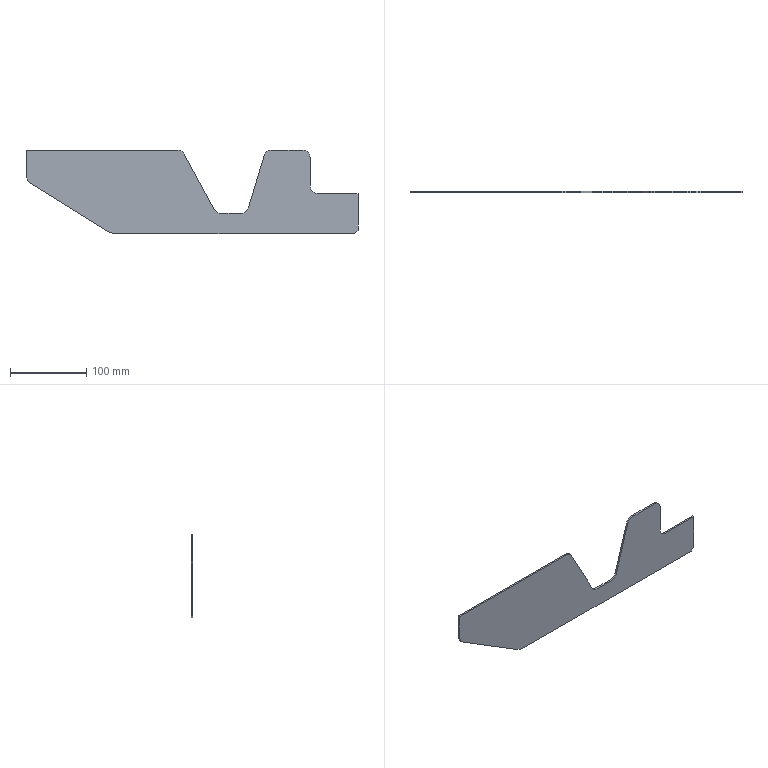Part | SolidWorks | features Chamfer 2, Fillet 1, FlatPattern 1, SMBaseFlange 1, SheetMetal 1 | 1 solid | 22 faces | box 436 x 2.3 x 110 mm | volume 78566 mm3 | plane 16 | cylinder 6 | commonest cylinder face diameters 20 x6
STEP:
#1=CARTESIAN_POINT('',(0.,0.,-35.));
#2=VERTEX_POINT('',#1);
#3=CARTESIAN_POINT('',(0.,0.,0.));
#4=VERTEX_POINT('',#3);
#5=CARTESIAN_POINT('',(0.,0.,-40.));
#6=DIRECTION('',(0.,0.,1.));
#7=VECTOR('',#6,1000.);
#8=LINE('',#5,#7);
#9=EDGE_CURVE('',#2,#4,#8,.T.);
#10=ORIENTED_EDGE('',*,*,#9,.F.);
#11=CARTESIAN_POINT('',(0.,-2.3,-35.));
#12=VERTEX_POINT('',#11);
#13=CARTESIAN_POINT('',(0.,-2.3,-35.));
#14=DIRECTION('',(0.,-1.,0.));
#15=VECTOR('',#14,1000.);
#16=LINE('',#13,#15);
#17=EDGE_CURVE('',#2,#12,#16,.T.);
#18=ORIENTED_EDGE('',*,*,#17,.T.);
#19=CARTESIAN_POINT('',(0.,-2.3,0.));
#20=VERTEX_POINT('',#19);
#21=CARTESIAN_POINT('',(0.,-2.3,-40.));
#22=DIRECTION('',(0.,0.,1.));
#23=VECTOR('',#22,1000.);
#24=LINE('',#21,#23);
#25=EDGE_CURVE('',#12,#20,#24,.T.);
#26=ORIENTED_EDGE('',*,*,#25,.T.);
#27=CARTESIAN_POINT('',(0.,-2.3,0.));
#28=DIRECTION('',(0.,1.,0.));
#29=VECTOR('',#28,1000.);
#30=LINE('',#27,#29);
#31=EDGE_CURVE('',#20,#4,#30,.T.);
#32=ORIENTED_EDGE('',*,*,#31,.T.);
#33=EDGE_LOOP('',(#10,#18,#26,#32));
#34=FACE_OUTER_BOUND('',#33,.T.);
#35=CARTESIAN_POINT('',(0.,-2.3,-40.));
#36=DIRECTION('',(-1.,0.,0.));
#37=DIRECTION('',(0.,0.,1.));
#38=AXIS2_PLACEMENT_3D('',#35,#36,#37);
#39=PLANE('',#38);
#40=ADVANCED_FACE('',(#34),#39,.T.);
#41=CARTESIAN_POINT('',(108.749,-2.3,-107.367));
#42=VERTEX_POINT('',#41);
#43=CARTESIAN_POINT('',(4.251,-2.3,-42.633));
#44=VERTEX_POINT('',#43);
#45=CARTESIAN_POINT('',(113.,-2.3,-110.));
#46=DIRECTION('',(-0.8501,0.,0.5266));
#47=VECTOR('',#46,1000.);
#48=LINE('',#45,#47);
#49=EDGE_CURVE('',#42,#44,#48,.T.);
#50=ORIENTED_EDGE('',*,*,#49,.T.);
#51=CARTESIAN_POINT('',(4.251,0.,-42.633));
#52=VERTEX_POINT('',#51);
#53=CARTESIAN_POINT('',(4.251,-2.3,-42.633));
#54=DIRECTION('',(0.,1.,0.));
#55=VECTOR('',#54,1000.);
#56=LINE('',#53,#55);
#57=EDGE_CURVE('',#44,#52,#56,.T.);
#58=ORIENTED_EDGE('',*,*,#57,.T.);
#59=CARTESIAN_POINT('',(108.749,0.,-107.367));
#60=VERTEX_POINT('',#59);
#61=CARTESIAN_POINT('',(113.,0.,-110.));
#62=DIRECTION('',(-0.8501,0.,0.5266));
#63=VECTOR('',#62,1000.);
#64=LINE('',#61,#63);
#65=EDGE_CURVE('',#60,#52,#64,.T.);
#66=ORIENTED_EDGE('',*,*,#65,.F.);
#67=CARTESIAN_POINT('',(108.749,-2.3,-107.367));
#68=DIRECTION('',(0.,-1.,0.));
#69=VECTOR('',#68,1000.);
#70=LINE('',#67,#69);
#71=EDGE_CURVE('',#60,#42,#70,.T.);
#72=ORIENTED_EDGE('',*,*,#71,.T.);
#73=EDGE_LOOP('',(#50,#58,#66,#72));
#74=FACE_OUTER_BOUND('',#73,.T.);
#75=CARTESIAN_POINT('',(113.,-2.3,-110.));
#76=DIRECTION('',(-0.5266,0.,-0.8501));
#77=DIRECTION('',(-0.8501,0.,0.5266));
#78=AXIS2_PLACEMENT_3D('',#75,#76,#77);
#79=PLANE('',#78);
#80=ADVANCED_FACE('',(#74),#79,.T.);
#81=CARTESIAN_POINT('',(431.,-2.3,-110.));
#82=VERTEX_POINT('',#81);
#83=CARTESIAN_POINT('',(118.,-2.3,-110.));
#84=VERTEX_POINT('',#83);
#85=CARTESIAN_POINT('',(436.,-2.3,-110.));
#86=DIRECTION('',(-1.,0.,0.));
#87=VECTOR('',#86,1000.);
#88=LINE('',#85,#87);
#89=EDGE_CURVE('',#82,#84,#88,.T.);
#90=ORIENTED_EDGE('',*,*,#89,.T.);
#91=CARTESIAN_POINT('',(118.,0.,-110.));
#92=VERTEX_POINT('',#91);
#93=CARTESIAN_POINT('',(118.,-2.3,-110.));
#94=DIRECTION('',(0.,1.,0.));
#95=VECTOR('',#94,1000.);
#96=LINE('',#93,#95);
#97=EDGE_CURVE('',#84,#92,#96,.T.);
#98=ORIENTED_EDGE('',*,*,#97,.T.);
#99=CARTESIAN_POINT('',(431.,0.,-110.));
#100=VERTEX_POINT('',#99);
#101=CARTESIAN_POINT('',(436.,0.,-110.));
#102=DIRECTION('',(-1.,0.,0.));
#103=VECTOR('',#102,1000.);
#104=LINE('',#101,#103);
#105=EDGE_CURVE('',#100,#92,#104,.T.);
#106=ORIENTED_EDGE('',*,*,#105,.F.);
#107=CARTESIAN_POINT('',(431.,-2.3,-110.));
#108=DIRECTION('',(0.,-1.,0.));
#109=VECTOR('',#108,1000.);
#110=LINE('',#107,#109);
#111=EDGE_CURVE('',#100,#82,#110,.T.);
#112=ORIENTED_EDGE('',*,*,#111,.T.);
#113=EDGE_LOOP('',(#90,#98,#106,#112));
#114=FACE_OUTER_BOUND('',#113,.T.);
#115=CARTESIAN_POINT('',(436.,-2.3,-110.));
#116=DIRECTION('',(0.,0.,-1.));
#117=DIRECTION('',(-1.,0.,0.));
#118=AXIS2_PLACEMENT_3D('',#115,#116,#117);
#119=PLANE('',#118);
#120=ADVANCED_FACE('',(#114),#119,.T.);
#121=CARTESIAN_POINT('',(436.,-2.3,-57.));
#122=VERTEX_POINT('',#121);
#123=CARTESIAN_POINT('',(436.,-2.3,-105.));
#124=VERTEX_POINT('',#123);
#125=CARTESIAN_POINT('',(436.,-2.3,-57.));
#126=DIRECTION('',(0.,0.,-1.));
#127=VECTOR('',#126,1000.);
#128=LINE('',#125,#127);
#129=EDGE_CURVE('',#122,#124,#128,.T.);
#130=ORIENTED_EDGE('',*,*,#129,.T.);
#131=CARTESIAN_POINT('',(436.,0.,-105.));
#132=VERTEX_POINT('',#131);
#133=CARTESIAN_POINT('',(436.,-2.3,-105.));
#134=DIRECTION('',(0.,1.,0.));
#135=VECTOR('',#134,1000.);
#136=LINE('',#133,#135);
#137=EDGE_CURVE('',#124,#132,#136,.T.);
#138=ORIENTED_EDGE('',*,*,#137,.T.);
#139=CARTESIAN_POINT('',(436.,0.,-57.));
#140=VERTEX_POINT('',#139);
#141=CARTESIAN_POINT('',(436.,0.,-57.));
#142=DIRECTION('',(0.,0.,-1.));
#143=VECTOR('',#142,1000.);
#144=LINE('',#141,#143);
#145=EDGE_CURVE('',#140,#132,#144,.T.);
#146=ORIENTED_EDGE('',*,*,#145,.F.);
#147=CARTESIAN_POINT('',(436.,-2.3,-57.));
#148=DIRECTION('',(0.,1.,0.));
#149=VECTOR('',#148,1000.);
#150=LINE('',#147,#149);
#151=EDGE_CURVE('',#122,#140,#150,.T.);
#152=ORIENTED_EDGE('',*,*,#151,.F.);
#153=EDGE_LOOP('',(#130,#138,#146,#152));
#154=FACE_OUTER_BOUND('',#153,.T.);
#155=CARTESIAN_POINT('',(436.,-2.3,-57.));
#156=DIRECTION('',(1.,0.,0.));
#157=DIRECTION('',(0.,0.,-1.));
#158=AXIS2_PLACEMENT_3D('',#155,#156,#157);
#159=PLANE('',#158);
#160=ADVANCED_FACE('',(#154),#159,.T.);
#161=CARTESIAN_POINT('',(383.,0.,-57.));
#162=VERTEX_POINT('',#161);
#163=CARTESIAN_POINT('',(373.,0.,-57.));
#164=DIRECTION('',(1.,0.,0.));
#165=VECTOR('',#164,1000.);
#166=LINE('',#163,#165);
#167=EDGE_CURVE('',#162,#140,#166,.T.);
#168=ORIENTED_EDGE('',*,*,#167,.F.);
#169=CARTESIAN_POINT('',(383.,-2.3,-57.));
#170=VERTEX_POINT('',#169);
#171=CARTESIAN_POINT('',(383.,-2.3,-57.));
#172=DIRECTION('',(0.,-1.,0.));
#173=VECTOR('',#172,1000.);
#174=LINE('',#171,#173);
#175=EDGE_CURVE('',#162,#170,#174,.T.);
#176=ORIENTED_EDGE('',*,*,#175,.T.);
#177=CARTESIAN_POINT('',(373.,-2.3,-57.));
#178=DIRECTION('',(1.,0.,0.));
#179=VECTOR('',#178,1000.);
#180=LINE('',#177,#179);
#181=EDGE_CURVE('',#170,#122,#180,.T.);
#182=ORIENTED_EDGE('',*,*,#181,.T.);
#183=ORIENTED_EDGE('',*,*,#151,.T.);
#184=EDGE_LOOP('',(#168,#176,#182,#183));
#185=FACE_OUTER_BOUND('',#184,.T.);
#186=CARTESIAN_POINT('',(373.,-2.3,-57.));
#187=DIRECTION('',(0.,0.,1.));
#188=DIRECTION('',(1.,0.,0.));
#189=AXIS2_PLACEMENT_3D('',#186,#187,#188);
#190=PLANE('',#189);
#191=ADVANCED_FACE('',(#185),#190,.T.);
#192=CARTESIAN_POINT('',(373.,-2.3,-10.));
#193=VERTEX_POINT('',#192);
#194=CARTESIAN_POINT('',(373.,-2.3,-47.));
#195=VERTEX_POINT('',#194);
#196=CARTESIAN_POINT('',(373.,-2.3,0.));
#197=DIRECTION('',(0.,0.,-1.));
#198=VECTOR('',#197,1000.);
#199=LINE('',#196,#198);
#200=EDGE_CURVE('',#193,#195,#199,.T.);
#201=ORIENTED_EDGE('',*,*,#200,.T.);
#202=CARTESIAN_POINT('',(373.,0.,-47.));
#203=VERTEX_POINT('',#202);
#204=CARTESIAN_POINT('',(373.,0.,-47.));
#205=DIRECTION('',(0.,1.,0.));
#206=VECTOR('',#205,1000.);
#207=LINE('',#204,#206);
#208=EDGE_CURVE('',#195,#203,#207,.T.);
#209=ORIENTED_EDGE('',*,*,#208,.T.);
#210=CARTESIAN_POINT('',(373.,0.,-10.));
#211=VERTEX_POINT('',#210);
#212=CARTESIAN_POINT('',(373.,0.,0.));
#213=DIRECTION('',(0.,0.,-1.));
#214=VECTOR('',#213,1000.);
#215=LINE('',#212,#214);
#216=EDGE_CURVE('',#211,#203,#215,.T.);
#217=ORIENTED_EDGE('',*,*,#216,.F.);
#218=CARTESIAN_POINT('',(373.,-2.3,-10.));
#219=DIRECTION('',(0.,-1.,0.));
#220=VECTOR('',#219,1000.);
#221=LINE('',#218,#220);
#222=EDGE_CURVE('',#211,#193,#221,.T.);
#223=ORIENTED_EDGE('',*,*,#222,.T.);
#224=EDGE_LOOP('',(#201,#209,#217,#223));
#225=FACE_OUTER_BOUND('',#224,.T.);
#226=CARTESIAN_POINT('',(373.,-2.3,0.));
#227=DIRECTION('',(1.,0.,0.));
#228=DIRECTION('',(0.,0.,-1.));
#229=AXIS2_PLACEMENT_3D('',#226,#227,#228);
#230=PLANE('',#229);
#231=ADVANCED_FACE('',(#225),#230,.T.);
#232=CARTESIAN_POINT('',(322.432,-2.3,0.));
#233=VERTEX_POINT('',#232);
#234=CARTESIAN_POINT('',(363.,-2.3,0.));
#235=VERTEX_POINT('',#234);
#236=CARTESIAN_POINT('',(315.,-2.3,0.));
#237=DIRECTION('',(1.,0.,0.));
#238=VECTOR('',#237,1000.);
#239=LINE('',#236,#238);
#240=EDGE_CURVE('',#233,#235,#239,.T.);
#241=ORIENTED_EDGE('',*,*,#240,.T.);
#242=CARTESIAN_POINT('',(363.,0.,0.));
#243=VERTEX_POINT('',#242);
#244=CARTESIAN_POINT('',(363.,-2.3,0.));
#245=DIRECTION('',(0.,1.,0.));
#246=VECTOR('',#245,1000.);
#247=LINE('',#244,#246);
#248=EDGE_CURVE('',#235,#243,#247,.T.);
#249=ORIENTED_EDGE('',*,*,#248,.T.);
#250=CARTESIAN_POINT('',(322.432,0.,0.));
#251=VERTEX_POINT('',#250);
#252=CARTESIAN_POINT('',(315.,0.,0.));
#253=DIRECTION('',(1.,0.,0.));
#254=VECTOR('',#253,1000.);
#255=LINE('',#252,#254);
#256=EDGE_CURVE('',#251,#243,#255,.T.);
#257=ORIENTED_EDGE('',*,*,#256,.F.);
#258=CARTESIAN_POINT('',(322.432,-2.3,0.));
#259=DIRECTION('',(0.,-1.,0.));
#260=VECTOR('',#259,1000.);
#261=LINE('',#258,#260);
#262=EDGE_CURVE('',#251,#233,#261,.T.);
#263=ORIENTED_EDGE('',*,*,#262,.T.);
#264=EDGE_LOOP('',(#241,#249,#257,#263));
#265=FACE_OUTER_BOUND('',#264,.T.);
#266=CARTESIAN_POINT('',(315.,-2.3,0.));
#267=DIRECTION('',(0.,0.,1.));
#268=DIRECTION('',(1.,0.,0.));
#269=AXIS2_PLACEMENT_3D('',#266,#267,#268);
#270=PLANE('',#269);
#271=ADVANCED_FACE('',(#265),#270,.T.);
#272=CARTESIAN_POINT('',(292.143,-2.3,-75.884));
#273=VERTEX_POINT('',#272);
#274=CARTESIAN_POINT('',(312.857,-2.3,-7.116));
#275=VERTEX_POINT('',#274);
#276=CARTESIAN_POINT('',(290.,-2.3,-83.));
#277=DIRECTION('',(0.2884,0.,0.9575));
#278=VECTOR('',#277,1000.);
#279=LINE('',#276,#278);
#280=EDGE_CURVE('',#273,#275,#279,.T.);
#281=ORIENTED_EDGE('',*,*,#280,.T.);
#282=CARTESIAN_POINT('',(312.857,0.,-7.116));
#283=VERTEX_POINT('',#282);
#284=CARTESIAN_POINT('',(312.857,-2.3,-7.116));
#285=DIRECTION('',(0.,1.,0.));
#286=VECTOR('',#285,1000.);
#287=LINE('',#284,#286);
#288=EDGE_CURVE('',#275,#283,#287,.T.);
#289=ORIENTED_EDGE('',*,*,#288,.T.);
#290=CARTESIAN_POINT('',(292.143,0.,-75.884));
#291=VERTEX_POINT('',#290);
#292=CARTESIAN_POINT('',(290.,0.,-83.));
#293=DIRECTION('',(0.2884,0.,0.9575));
#294=VECTOR('',#293,1000.);
#295=LINE('',#292,#294);
#296=EDGE_CURVE('',#291,#283,#295,.T.);
#297=ORIENTED_EDGE('',*,*,#296,.F.);
#298=CARTESIAN_POINT('',(292.143,-2.3,-75.884));
#299=DIRECTION('',(0.,-1.,0.));
#300=VECTOR('',#299,1000.);
#301=LINE('',#298,#300);
#302=EDGE_CURVE('',#291,#273,#301,.T.);
#303=ORIENTED_EDGE('',*,*,#302,.T.);
#304=EDGE_LOOP('',(#281,#289,#297,#303));
#305=FACE_OUTER_BOUND('',#304,.T.);
#306=CARTESIAN_POINT('',(290.,-2.3,-83.));
#307=DIRECTION('',(-0.9575,0.,0.2884));
#308=DIRECTION('',(0.2884,0.,0.9575));
#309=AXIS2_PLACEMENT_3D('',#306,#307,#308);
#310=PLANE('',#309);
#311=ADVANCED_FACE('',(#305),#310,.T.);
#312=CARTESIAN_POINT('',(255.953,-2.3,-83.));
#313=VERTEX_POINT('',#312);
#314=CARTESIAN_POINT('',(282.568,-2.3,-83.));
#315=VERTEX_POINT('',#314);
#316=CARTESIAN_POINT('',(250.,-2.3,-83.));
#317=DIRECTION('',(1.,0.,0.));
#318=VECTOR('',#317,1000.);
#319=LINE('',#316,#318);
#320=EDGE_CURVE('',#313,#315,#319,.T.);
#321=ORIENTED_EDGE('',*,*,#320,.T.);
#322=CARTESIAN_POINT('',(282.568,0.,-83.));
#323=VERTEX_POINT('',#322);
#324=CARTESIAN_POINT('',(282.568,0.,-83.));
#325=DIRECTION('',(0.,1.,0.));
#326=VECTOR('',#325,1000.);
#327=LINE('',#324,#326);
#328=EDGE_CURVE('',#315,#323,#327,.T.);
#329=ORIENTED_EDGE('',*,*,#328,.T.);
#330=CARTESIAN_POINT('',(255.953,0.,-83.));
#331=VERTEX_POINT('',#330);
#332=CARTESIAN_POINT('',(250.,0.,-83.));
#333=DIRECTION('',(1.,0.,0.));
#334=VECTOR('',#333,1000.);
#335=LINE('',#332,#334);
#336=EDGE_CURVE('',#331,#323,#335,.T.);
#337=ORIENTED_EDGE('',*,*,#336,.F.);
#338=CARTESIAN_POINT('',(255.953,-2.3,-83.));
#339=DIRECTION('',(0.,-1.,0.));
#340=VECTOR('',#339,1000.);
#341=LINE('',#338,#340);
#342=EDGE_CURVE('',#331,#313,#341,.T.);
#343=ORIENTED_EDGE('',*,*,#342,.T.);
#344=EDGE_LOOP('',(#321,#329,#337,#343));
#345=FACE_OUTER_BOUND('',#344,.T.);
#346=CARTESIAN_POINT('',(250.,-2.3,-83.));
#347=DIRECTION('',(0.,0.,1.));
#348=DIRECTION('',(1.,0.,0.));
#349=AXIS2_PLACEMENT_3D('',#346,#347,#348);
#350=PLANE('',#349);
#351=ADVANCED_FACE('',(#345),#350,.T.);
#352=CARTESIAN_POINT('',(207.838,-2.3,-5.234));
#353=VERTEX_POINT('',#352);
#354=CARTESIAN_POINT('',(247.162,-2.3,-77.766));
#355=VERTEX_POINT('',#354);
#356=CARTESIAN_POINT('',(205.,-2.3,0.));
#357=DIRECTION('',(0.4766,0.,-0.8791));
#358=VECTOR('',#357,1000.);
#359=LINE('',#356,#358);
#360=EDGE_CURVE('',#353,#355,#359,.T.);
#361=ORIENTED_EDGE('',*,*,#360,.T.);
#362=CARTESIAN_POINT('',(247.162,0.,-77.766));
#363=VERTEX_POINT('',#362);
#364=CARTESIAN_POINT('',(247.162,0.,-77.766));
#365=DIRECTION('',(0.,1.,0.));
#366=VECTOR('',#365,1000.);
#367=LINE('',#364,#366);
#368=EDGE_CURVE('',#355,#363,#367,.T.);
#369=ORIENTED_EDGE('',*,*,#368,.T.);
#370=CARTESIAN_POINT('',(207.838,0.,-5.234));
#371=VERTEX_POINT('',#370);
#372=CARTESIAN_POINT('',(205.,0.,0.));
#373=DIRECTION('',(0.4766,0.,-0.8791));
#374=VECTOR('',#373,1000.);
#375=LINE('',#372,#374);
#376=EDGE_CURVE('',#371,#363,#375,.T.);
#377=ORIENTED_EDGE('',*,*,#376,.F.);
#378=CARTESIAN_POINT('',(207.838,-2.3,-5.234));
#379=DIRECTION('',(0.,-1.,0.));
#380=VECTOR('',#379,1000.);
#381=LINE('',#378,#380);
#382=EDGE_CURVE('',#371,#353,#381,.T.);
#383=ORIENTED_EDGE('',*,*,#382,.T.);
#384=EDGE_LOOP('',(#361,#369,#377,#383));
#385=FACE_OUTER_BOUND('',#384,.T.);
#386=CARTESIAN_POINT('',(205.,-2.3,0.));
#387=DIRECTION('',(0.8791,0.,0.4766));
#388=DIRECTION('',(0.4766,0.,-0.8791));
#389=AXIS2_PLACEMENT_3D('',#386,#387,#388);
#390=PLANE('',#389);
#391=ADVANCED_FACE('',(#385),#390,.T.);
#392=CARTESIAN_POINT('',(199.047,-2.3,0.));
#393=VERTEX_POINT('',#392);
#394=CARTESIAN_POINT('',(0.,-2.3,0.));
#395=DIRECTION('',(1.,0.,0.));
#396=VECTOR('',#395,1000.);
#397=LINE('',#394,#396);
#398=EDGE_CURVE('',#20,#393,#397,.T.);
#399=ORIENTED_EDGE('',*,*,#398,.T.);
#400=CARTESIAN_POINT('',(199.047,0.,0.));
#401=VERTEX_POINT('',#400);
#402=CARTESIAN_POINT('',(199.047,-2.3,0.));
#403=DIRECTION('',(0.,1.,0.));
#404=VECTOR('',#403,1000.);
#405=LINE('',#402,#404);
#406=EDGE_CURVE('',#393,#401,#405,.T.);
#407=ORIENTED_EDGE('',*,*,#406,.T.);
#408=CARTESIAN_POINT('',(0.,0.,0.));
#409=DIRECTION('',(1.,0.,0.));
#410=VECTOR('',#409,1000.);
#411=LINE('',#408,#410);
#412=EDGE_CURVE('',#4,#401,#411,.T.);
#413=ORIENTED_EDGE('',*,*,#412,.F.);
#414=ORIENTED_EDGE('',*,*,#31,.F.);
#415=EDGE_LOOP('',(#399,#407,#413,#414));
#416=FACE_OUTER_BOUND('',#415,.T.);
#417=CARTESIAN_POINT('',(0.,-2.3,0.));
#418=DIRECTION('',(0.,0.,1.));
#419=DIRECTION('',(1.,0.,0.));
#420=AXIS2_PLACEMENT_3D('',#417,#418,#419);
#421=PLANE('',#420);
#422=ADVANCED_FACE('',(#416),#421,.T.);
#423=ORIENTED_EDGE('',*,*,#25,.F.);
#424=CARTESIAN_POINT('',(4.251,-2.3,-42.633));
#425=DIRECTION('',(0.4865,0.,-0.8737));
#426=VECTOR('',#425,1000.);
#427=LINE('',#424,#426);
#428=EDGE_CURVE('',#12,#44,#427,.T.);
#429=ORIENTED_EDGE('',*,*,#428,.T.);
#430=ORIENTED_EDGE('',*,*,#49,.F.);
#431=CARTESIAN_POINT('',(118.,-2.3,-110.));
#432=DIRECTION('',(0.9618,0.,-0.2738));
#433=VECTOR('',#432,1000.);
#434=LINE('',#431,#433);
#435=EDGE_CURVE('',#42,#84,#434,.T.);
#436=ORIENTED_EDGE('',*,*,#435,.T.);
#437=ORIENTED_EDGE('',*,*,#89,.F.);
#438=CARTESIAN_POINT('',(436.,-2.3,-105.));
#439=DIRECTION('',(0.7071,0.,0.7071));
#440=VECTOR('',#439,1000.);
#441=LINE('',#438,#440);
#442=EDGE_CURVE('',#82,#124,#441,.T.);
#443=ORIENTED_EDGE('',*,*,#442,.T.);
#444=ORIENTED_EDGE('',*,*,#129,.F.);
#445=ORIENTED_EDGE('',*,*,#181,.F.);
#446=CARTESIAN_POINT('',(383.,-2.3,-47.));
#447=DIRECTION('',(0.,1.,0.));
#448=DIRECTION('',(0.,0.,1.));
#449=AXIS2_PLACEMENT_3D('',#446,#447,#448);
#450=CIRCLE('',#449,10.);
#451=EDGE_CURVE('',#170,#195,#450,.T.);
#452=ORIENTED_EDGE('',*,*,#451,.T.);
#453=ORIENTED_EDGE('',*,*,#200,.F.);
#454=CARTESIAN_POINT('',(363.,-2.3,-10.));
#455=DIRECTION('',(0.,-1.,0.));
#456=DIRECTION('',(0.,0.,1.));
#457=AXIS2_PLACEMENT_3D('',#454,#455,#456);
#458=CIRCLE('',#457,10.);
#459=EDGE_CURVE('',#193,#235,#458,.T.);
#460=ORIENTED_EDGE('',*,*,#459,.T.);
#461=ORIENTED_EDGE('',*,*,#240,.F.);
#462=CARTESIAN_POINT('',(322.432,-2.3,-10.));
#463=DIRECTION('',(0.,-1.,0.));
#464=DIRECTION('',(0.,0.,1.));
#465=AXIS2_PLACEMENT_3D('',#462,#463,#464);
#466=CIRCLE('',#465,10.);
#467=EDGE_CURVE('',#233,#275,#466,.T.);
#468=ORIENTED_EDGE('',*,*,#467,.T.);
#469=ORIENTED_EDGE('',*,*,#280,.F.);
#470=CARTESIAN_POINT('',(282.568,-2.3,-73.));
#471=DIRECTION('',(0.,1.,0.));
#472=DIRECTION('',(0.,0.,1.));
#473=AXIS2_PLACEMENT_3D('',#470,#471,#472);
#474=CIRCLE('',#473,10.);
#475=EDGE_CURVE('',#273,#315,#474,.T.);
#476=ORIENTED_EDGE('',*,*,#475,.T.);
#477=ORIENTED_EDGE('',*,*,#320,.F.);
#478=CARTESIAN_POINT('',(255.953,-2.3,-73.));
#479=DIRECTION('',(0.,1.,0.));
#480=DIRECTION('',(0.,0.,1.));
#481=AXIS2_PLACEMENT_3D('',#478,#479,#480);
#482=CIRCLE('',#481,10.);
#483=EDGE_CURVE('',#313,#355,#482,.T.);
#484=ORIENTED_EDGE('',*,*,#483,.T.);
#485=ORIENTED_EDGE('',*,*,#360,.F.);
#486=CARTESIAN_POINT('',(199.047,-2.3,-10.));
#487=DIRECTION('',(0.,-1.,0.));
#488=DIRECTION('',(0.,0.,1.));
#489=AXIS2_PLACEMENT_3D('',#486,#487,#488);
#490=CIRCLE('',#489,10.);
#491=EDGE_CURVE('',#353,#393,#490,.T.);
#492=ORIENTED_EDGE('',*,*,#491,.T.);
#493=ORIENTED_EDGE('',*,*,#398,.F.);
#494=EDGE_LOOP('',(#423,#429,#430,#436,#437,#443,#444,#445,#452,#453,#460,#461,#468,#469,#476,#477,#484,#485,#492,#493));
#495=FACE_OUTER_BOUND('',#494,.T.);
#496=CARTESIAN_POINT('',(0.,-2.3,0.));
#497=DIRECTION('',(0.,1.,0.));
#498=DIRECTION('',(0.,0.,1.));
#499=AXIS2_PLACEMENT_3D('',#496,#497,#498);
#500=PLANE('',#499);
#501=ADVANCED_FACE('',(#495),#500,.F.);
#502=ORIENTED_EDGE('',*,*,#65,.T.);
#503=CARTESIAN_POINT('',(-14.877,0.,-8.284));
#504=DIRECTION('',(-0.4865,0.,0.8737));
#505=VECTOR('',#504,1000.);
#506=LINE('',#503,#505);
#507=EDGE_CURVE('',#52,#2,#506,.T.);
#508=ORIENTED_EDGE('',*,*,#507,.T.);
#509=ORIENTED_EDGE('',*,*,#9,.T.);
#510=ORIENTED_EDGE('',*,*,#412,.T.);
#511=CARTESIAN_POINT('',(199.047,0.,-10.));
#512=DIRECTION('',(0.,1.,0.));
#513=DIRECTION('',(0.,0.,1.));
#514=AXIS2_PLACEMENT_3D('',#511,#512,#513);
#515=CIRCLE('',#514,10.);
#516=EDGE_CURVE('',#401,#371,#515,.T.);
#517=ORIENTED_EDGE('',*,*,#516,.T.);
#518=ORIENTED_EDGE('',*,*,#376,.T.);
#519=CARTESIAN_POINT('',(255.953,0.,-73.));
#520=DIRECTION('',(0.,-1.,0.));
#521=DIRECTION('',(0.,0.,1.));
#522=AXIS2_PLACEMENT_3D('',#519,#520,#521);
#523=CIRCLE('',#522,10.);
#524=EDGE_CURVE('',#363,#331,#523,.T.);
#525=ORIENTED_EDGE('',*,*,#524,.T.);
#526=ORIENTED_EDGE('',*,*,#336,.T.);
#527=CARTESIAN_POINT('',(282.568,0.,-73.));
#528=DIRECTION('',(0.,-1.,0.));
#529=DIRECTION('',(0.,0.,1.));
#530=AXIS2_PLACEMENT_3D('',#527,#528,#529);
#531=CIRCLE('',#530,10.);
#532=EDGE_CURVE('',#323,#291,#531,.T.);
#533=ORIENTED_EDGE('',*,*,#532,.T.);
#534=ORIENTED_EDGE('',*,*,#296,.T.);
#535=CARTESIAN_POINT('',(322.432,0.,-10.));
#536=DIRECTION('',(0.,1.,0.));
#537=DIRECTION('',(0.,0.,1.));
#538=AXIS2_PLACEMENT_3D('',#535,#536,#537);
#539=CIRCLE('',#538,10.);
#540=EDGE_CURVE('',#283,#251,#539,.T.);
#541=ORIENTED_EDGE('',*,*,#540,.T.);
#542=ORIENTED_EDGE('',*,*,#256,.T.);
#543=CARTESIAN_POINT('',(363.,0.,-10.));
#544=DIRECTION('',(0.,1.,0.));
#545=DIRECTION('',(0.,0.,1.));
#546=AXIS2_PLACEMENT_3D('',#543,#544,#545);
#547=CIRCLE('',#546,10.);
#548=EDGE_CURVE('',#243,#211,#547,.T.);
#549=ORIENTED_EDGE('',*,*,#548,.T.);
#550=ORIENTED_EDGE('',*,*,#216,.T.);
#551=CARTESIAN_POINT('',(383.,0.,-47.));
#552=DIRECTION('',(0.,-1.,0.));
#553=DIRECTION('',(0.,0.,1.));
#554=AXIS2_PLACEMENT_3D('',#551,#552,#553);
#555=CIRCLE('',#554,10.);
#556=EDGE_CURVE('',#203,#162,#555,.T.);
#557=ORIENTED_EDGE('',*,*,#556,.T.);
#558=ORIENTED_EDGE('',*,*,#167,.T.);
#559=ORIENTED_EDGE('',*,*,#145,.T.);
#560=CARTESIAN_POINT('',(270.5,0.,-270.5));
#561=DIRECTION('',(-0.7071,0.,-0.7071));
#562=VECTOR('',#561,1000.);
#563=LINE('',#560,#562);
#564=EDGE_CURVE('',#132,#100,#563,.T.);
#565=ORIENTED_EDGE('',*,*,#564,.T.);
#566=ORIENTED_EDGE('',*,*,#105,.T.);
#567=CARTESIAN_POINT('',(-20.12,0.,-70.686));
#568=DIRECTION('',(-0.9618,0.,0.2738));
#569=VECTOR('',#568,1000.);
#570=LINE('',#567,#569);
#571=EDGE_CURVE('',#92,#60,#570,.T.);
#572=ORIENTED_EDGE('',*,*,#571,.T.);
#573=EDGE_LOOP('',(#502,#508,#509,#510,#517,#518,#525,#526,#533,#534,#541,#542,#549,#550,#557,#558,#559,#565,#566,#572));
#574=FACE_OUTER_BOUND('',#573,.T.);
#575=CARTESIAN_POINT('',(0.,0.,0.));
#576=DIRECTION('',(0.,1.,0.));
#577=DIRECTION('',(0.,0.,1.));
#578=AXIS2_PLACEMENT_3D('',#575,#576,#577);
#579=PLANE('',#578);
#580=ADVANCED_FACE('',(#574),#579,.T.);
#581=ORIENTED_EDGE('',*,*,#451,.F.);
#582=ORIENTED_EDGE('',*,*,#175,.F.);
#583=ORIENTED_EDGE('',*,*,#556,.F.);
#584=ORIENTED_EDGE('',*,*,#208,.F.);
#585=EDGE_LOOP('',(#581,#582,#583,#584));
#586=FACE_OUTER_BOUND('',#585,.T.);
#587=CARTESIAN_POINT('',(383.,-2.3,-47.));
#588=DIRECTION('',(0.,-1.,0.));
#589=DIRECTION('',(0.,0.,-1.));
#590=AXIS2_PLACEMENT_3D('',#587,#588,#589);
#591=CYLINDRICAL_SURFACE('',#590,10.);
#592=ADVANCED_FACE('',(#586),#591,.F.);
#593=ORIENTED_EDGE('',*,*,#459,.F.);
#594=ORIENTED_EDGE('',*,*,#222,.F.);
#595=ORIENTED_EDGE('',*,*,#548,.F.);
#596=ORIENTED_EDGE('',*,*,#248,.F.);
#597=EDGE_LOOP('',(#593,#594,#595,#596));
#598=FACE_OUTER_BOUND('',#597,.T.);
#599=CARTESIAN_POINT('',(363.,-2.3,-10.));
#600=DIRECTION('',(0.,1.,0.));
#601=DIRECTION('',(0.,0.,1.));
#602=AXIS2_PLACEMENT_3D('',#599,#600,#601);
#603=CYLINDRICAL_SURFACE('',#602,10.);
#604=ADVANCED_FACE('',(#598),#603,.T.);
#605=ORIENTED_EDGE('',*,*,#467,.F.);
#606=ORIENTED_EDGE('',*,*,#262,.F.);
#607=ORIENTED_EDGE('',*,*,#540,.F.);
#608=ORIENTED_EDGE('',*,*,#288,.F.);
#609=EDGE_LOOP('',(#605,#606,#607,#608));
#610=FACE_OUTER_BOUND('',#609,.T.);
#611=CARTESIAN_POINT('',(322.432,-2.3,-10.));
#612=DIRECTION('',(0.,1.,0.));
#613=DIRECTION('',(0.,0.,1.));
#614=AXIS2_PLACEMENT_3D('',#611,#612,#613);
#615=CYLINDRICAL_SURFACE('',#614,10.);
#616=ADVANCED_FACE('',(#610),#615,.T.);
#617=ORIENTED_EDGE('',*,*,#475,.F.);
#618=ORIENTED_EDGE('',*,*,#302,.F.);
#619=ORIENTED_EDGE('',*,*,#532,.F.);
#620=ORIENTED_EDGE('',*,*,#328,.F.);
#621=EDGE_LOOP('',(#617,#618,#619,#620));
#622=FACE_OUTER_BOUND('',#621,.T.);
#623=CARTESIAN_POINT('',(282.568,-2.3,-73.));
#624=DIRECTION('',(0.,-1.,0.));
#625=DIRECTION('',(0.,0.,-1.));
#626=AXIS2_PLACEMENT_3D('',#623,#624,#625);
#627=CYLINDRICAL_SURFACE('',#626,10.);
#628=ADVANCED_FACE('',(#622),#627,.F.);
#629=ORIENTED_EDGE('',*,*,#483,.F.);
#630=ORIENTED_EDGE('',*,*,#342,.F.);
#631=ORIENTED_EDGE('',*,*,#524,.F.);
#632=ORIENTED_EDGE('',*,*,#368,.F.);
#633=EDGE_LOOP('',(#629,#630,#631,#632));
#634=FACE_OUTER_BOUND('',#633,.T.);
#635=CARTESIAN_POINT('',(255.953,-2.3,-73.));
#636=DIRECTION('',(0.,-1.,0.));
#637=DIRECTION('',(0.,0.,-1.));
#638=AXIS2_PLACEMENT_3D('',#635,#636,#637);
#639=CYLINDRICAL_SURFACE('',#638,10.);
#640=ADVANCED_FACE('',(#634),#639,.F.);
#641=ORIENTED_EDGE('',*,*,#491,.F.);
#642=ORIENTED_EDGE('',*,*,#382,.F.);
#643=ORIENTED_EDGE('',*,*,#516,.F.);
#644=ORIENTED_EDGE('',*,*,#406,.F.);
#645=EDGE_LOOP('',(#641,#642,#643,#644));
#646=FACE_OUTER_BOUND('',#645,.T.);
#647=CARTESIAN_POINT('',(199.047,-2.3,-10.));
#648=DIRECTION('',(0.,1.,0.));
#649=DIRECTION('',(0.,0.,1.));
#650=AXIS2_PLACEMENT_3D('',#647,#648,#649);
#651=CYLINDRICAL_SURFACE('',#650,10.);
#652=ADVANCED_FACE('',(#646),#651,.T.);
#653=ORIENTED_EDGE('',*,*,#442,.F.);
#654=ORIENTED_EDGE('',*,*,#111,.F.);
#655=ORIENTED_EDGE('',*,*,#564,.F.);
#656=ORIENTED_EDGE('',*,*,#137,.F.);
#657=EDGE_LOOP('',(#653,#654,#655,#656));
#658=FACE_OUTER_BOUND('',#657,.T.);
#659=CARTESIAN_POINT('',(436.,-2.3,-105.));
#660=DIRECTION('',(-0.7071,0.,0.7071));
#661=DIRECTION('',(0.,1.,0.));
#662=AXIS2_PLACEMENT_3D('',#659,#660,#661);
#663=PLANE('',#662);
#664=ADVANCED_FACE('',(#658),#663,.F.);
#665=ORIENTED_EDGE('',*,*,#428,.F.);
#666=ORIENTED_EDGE('',*,*,#17,.F.);
#667=ORIENTED_EDGE('',*,*,#507,.F.);
#668=ORIENTED_EDGE('',*,*,#57,.F.);
#669=EDGE_LOOP('',(#665,#666,#667,#668));
#670=FACE_OUTER_BOUND('',#669,.T.);
#671=CARTESIAN_POINT('',(4.251,-2.3,-42.633));
#672=DIRECTION('',(0.8737,0.,0.4865));
#673=DIRECTION('',(0.,1.,0.));
#674=AXIS2_PLACEMENT_3D('',#671,#672,#673);
#675=PLANE('',#674);
#676=ADVANCED_FACE('',(#670),#675,.F.);
#677=ORIENTED_EDGE('',*,*,#435,.F.);
#678=ORIENTED_EDGE('',*,*,#71,.F.);
#679=ORIENTED_EDGE('',*,*,#571,.F.);
#680=ORIENTED_EDGE('',*,*,#97,.F.);
#681=EDGE_LOOP('',(#677,#678,#679,#680));
#682=FACE_OUTER_BOUND('',#681,.T.);
#683=CARTESIAN_POINT('',(118.,-2.3,-110.));
#684=DIRECTION('',(0.2738,0.,0.9618));
#685=DIRECTION('',(0.,1.,0.));
#686=AXIS2_PLACEMENT_3D('',#683,#684,#685);
#687=PLANE('',#686);
#688=ADVANCED_FACE('',(#682),#687,.F.);
#689=CLOSED_SHELL('',(#40,#80,#120,#160,#191,#231,#271,#311,#351,#391,#422,#501,#580,#592,#604,#616,#628,#640,#652,#664,#676,#688));
#690=MANIFOLD_SOLID_BREP('',#689);
#691=CARTESIAN_POINT('',(0.,0.,0.));
#692=DIRECTION('',(0.,0.,1.));
#693=DIRECTION('',(1.,0.,0.));
#694=AXIS2_PLACEMENT_3D('',#691,#692,#693);
#695=(LENGTH_UNIT()NAMED_UNIT(*)SI_UNIT(.MILLI.,.METRE.));
#696=UNCERTAINTY_MEASURE_WITH_UNIT(LENGTH_MEASURE(0.00001),#695,'','');
#697=(NAMED_UNIT(*)PLANE_ANGLE_UNIT()SI_UNIT($,.RADIAN.));
#698=(NAMED_UNIT(*)SI_UNIT($,.STERADIAN.)SOLID_ANGLE_UNIT());
#699=(GEOMETRIC_REPRESENTATION_CONTEXT(3)GLOBAL_UNCERTAINTY_ASSIGNED_CONTEXT((#696))GLOBAL_UNIT_ASSIGNED_CONTEXT((#695,#697,#698))REPRESENTATION_CONTEXT('',''));
#700=ADVANCED_BREP_SHAPE_REPRESENTATION('',(#690,#694),#699);